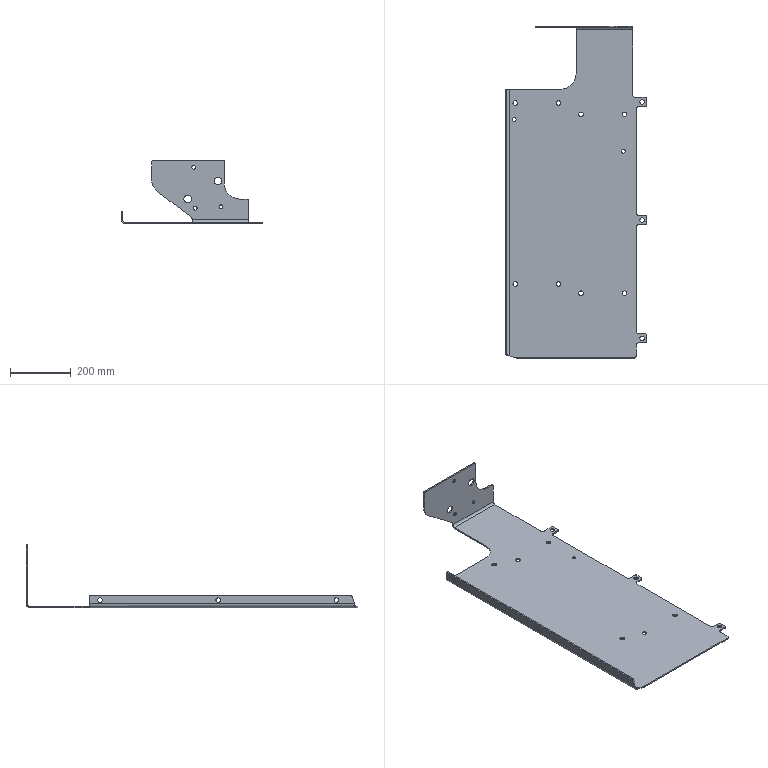Part | SolidWorks | features ICE 3, EdgeFlange 2, Fillet 2, FlatPattern 1, Fold 1, SMBaseFlange 1, SheetMetal 1, UnFold 1 | 1 solid | 106 faces | box 466 x 1095 x 209 mm | volume 2221279 mm3 | cylinder 69 | plane 36 | spline 1 | commonest cylinder face diameters 15 x28 10 x14 12.5 x10 20 x6 25 x6 100 x3